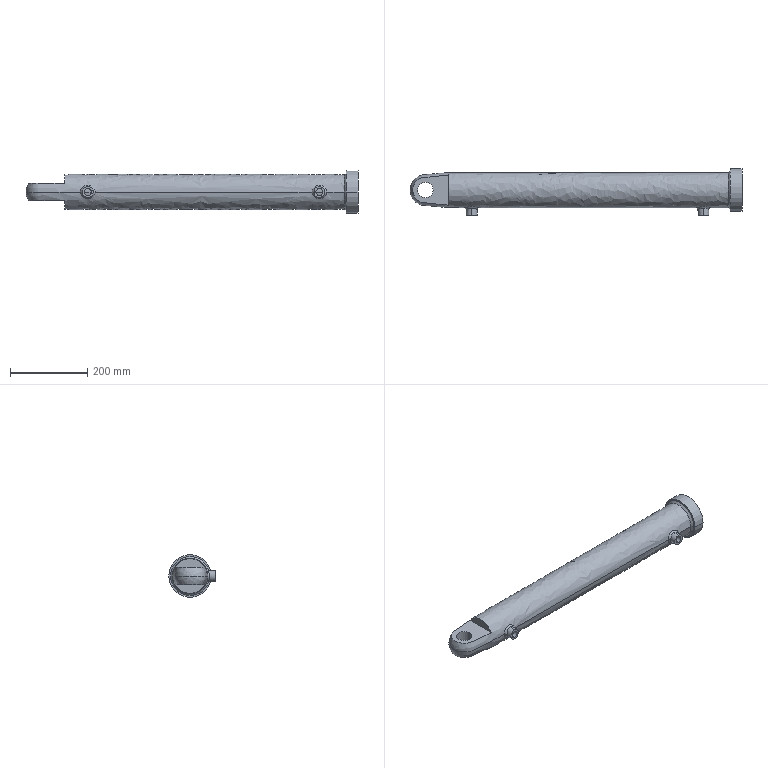Part | SolidWorks | features BaseBody 1 | 1 solid | 35 faces | box 860 x 120 x 110 mm | volume 3954634 mm3 | cylinder 14 | spline 10 | plane 9 | cone 2 | commonest cylinder face diameters 18 x4 28 x4 40 x2 50 x2 110 x2